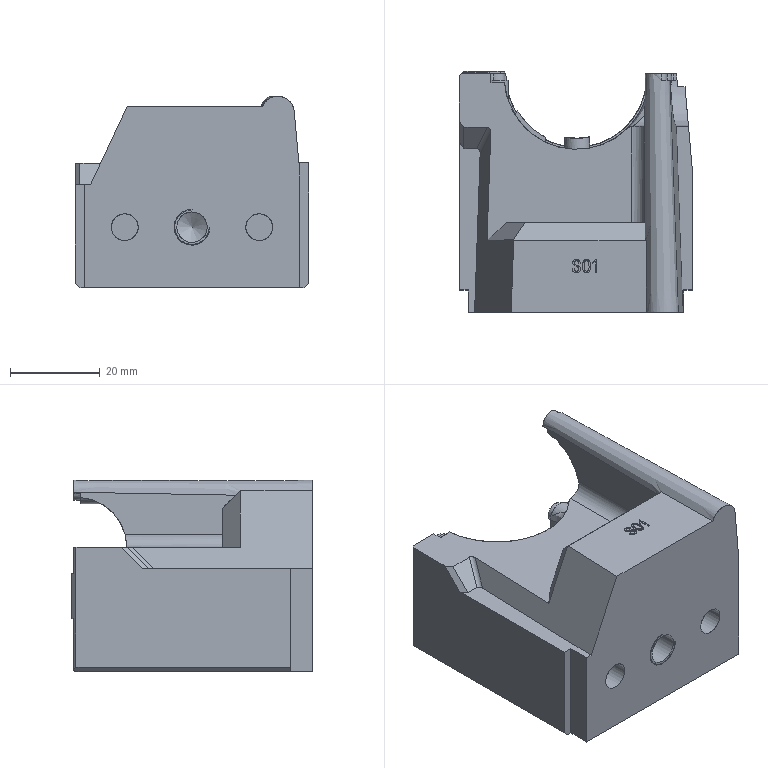NC program | PowerMill | posted with a generic post | part box 52 x 53.756 x 42.711 mm
Lines 1 to 741 of 2084:
%
O0001
N104 ( POWERMILL CB  : 2026004.0)
N105 ( POST VER      : 2026.0.0.5161)
N106 ( OPTION FILE   : FANUC)
N107 ( OUTPUT WORKPLANE : 3)
N108 (  )
N109 ( TOOL LIST )
N110 (----------------------------------)
N111 ( NO. | ID   | DIA.| TIP RAD|LENGTH)
N112 (----------------------------------)
N113 (    1|D4_1_1| 4.0 |  0.0   |108.56)
N114 (----------------------------------)
N115 (  )
N116 ( NUMBER OF TOOLPATHS: 1.0 )
N117 ( ESTIMATED PROGRAM DURATION: 0 HOURS 0 MIN 30 SEC)
N118 (  )
N119 G00 G21 G80 G40 G17
N120 G90
N121 G54
N122 G53 Z0.0
N123 (---------------)
N124 ( START TOOLPATH : 18开粗-D4-等高 )
N125 (---------------)
N126 ( TOOL NO.    :1 )
N127 ( TOOL TYPE   : ENDMILL)
N128 ( TOOL ID     : D4_1_1)
N129 ( TOOL DIA    : 4.0 LENGTH 108.56)
N130 T1
N131 M6
N132 S5500 M03
N133 G00 G90 X-25.2597 Y38.9756
N134 G43 Z63.21 H1
N135
N136 G05 P10000 R8
N137 Z30.842
N138 G01 Z27.842 F1800.0
N139 G02 X-24.8595 Y39.082 I0.3987 J-0.6936 F3000.0
N140 G01 X-21.6418 Y39.0761
N141 G02 X-21.2418 Y38.6655 I0.0002 J-0.4
N142 G01 X-21.362 Y35.186
N143 G02 X-21.483 Y34.7899 I-0.7996 J0.0276
N144 G01 X-21.512 Y34.7433
N145 X-21.5257 Y34.7207 Z27.8377
N146 X-21.5374 Y34.7001 Z27.8252
N147 X-21.5582 Y34.6616 Z27.7921
N148 X-21.561 Y34.6521 Z27.7611
N149 X-21.5457 Y34.6737 Z27.7422
N150 G03 X-21.4246 Y35.0697 I-0.6784 J0.4239
N151 G01 X-21.3028 Y38.5581
N152 G03 X-21.7026 Y38.9721 I-0.3998 J0.014
N153 G01 X-24.9911 Y38.9748
N154 G03 X-25.3912 Y38.8679 I-0.0006 J-0.8
N155 G01 X-25.4333 Y38.8436
N156 X-25.4578 Y38.8268 Z27.7371
N157 X-25.4764 Y38.8082 Z27.7225
N158 X-25.5002 Y38.7783 Z27.6923
N159 X-25.4996 Y38.7617 Z27.6607
N160 X-25.4697 Y38.7691 Z27.6424
N161 G02 X-25.0696 Y38.8758 I0.3992 J-0.6932
N162 G01 X-21.7526 Y38.8723
N163 G02 X-21.3529 Y38.4583 I0.0 J-0.4
N164 G01 X-21.4751 Y34.9589
N165 G02 X-21.5961 Y34.5629 I-0.7995 J0.0279
N166 G01 X-21.621 Y34.523
N167 X-21.6348 Y34.4999 Z27.6375
N168 X-21.6458 Y34.4792 Z27.6235
N169 X-21.6613 Y34.4474 Z27.5925
N170 X-21.6623 Y34.4389 Z27.5611
N171 X-21.6463 Y34.4605 Z27.5426
N172 G03 X-21.5252 Y34.8565 I-0.6784 J0.4239
N173 G01 X-21.4029 Y38.3585
N174 G03 X-21.8027 Y38.7725 I-0.3998 J0.014
N175 G01 X-25.1457 Y38.778
N176 G03 X-25.5459 Y38.6715 I-0.0013 J-0.8
N177 G01 X-25.5709 Y38.6571
N178 X-25.5973 Y38.6444 Z27.5356
N179 X-25.6195 Y38.6384 Z27.5163
N180 X-25.6379 Y38.6364 Z27.4921
N181 X-25.6424 Y38.641 Z27.4598
N182 X-25.6171 Y38.6535 Z27.4428
N183 G02 X-25.2045 Y38.689 I0.2727 J-0.7521
N184 G01 X-25.1367 Y38.677
N185 X-21.8527 Y38.6727
N186 G02 X-21.4529 Y38.2587 I0.0 J-0.4
N187 G01 X-21.5753 Y34.7559
N188 G02 X-21.6963 Y34.3599 I-0.7995 J0.0279
N189 G01 X-21.7209 Y34.3205
N190 X-21.7347 Y34.2975 Z27.4379
N191 X-21.7458 Y34.2769 Z27.4237
N192 X-21.7612 Y34.2458 Z27.3929
N193 X-21.7624 Y34.2375 Z27.3614
N194 X-21.7464 Y34.2592 Z27.343
N195 G03 X-21.6253 Y34.6552 I-0.6785 J0.424
N196 G01 X-21.503 Y38.1589
N197 G03 X-21.9028 Y38.5729 I-0.3997 J0.014
N198 G01 X-25.1367 Y38.5772
N199 X-25.2536 Y38.5993
N200 G03 X-25.6665 Y38.5684 I-0.1488 J-0.786
N201 G01 X-25.6952 Y38.5584
N202 X-25.7259 Y38.5425 Z27.3355
N203 X-25.7455 Y38.5215 Z27.3149
N204 X-25.7556 Y38.5031 Z27.2933
N205 X-25.749 Y38.4824 Z27.26
N206 X-25.713 Y38.483 Z27.2433
N207 G02 X-25.2997 Y38.5099 I0.2568 J-0.7577
N208 G01 X-25.1367 Y38.4774
N209 X-21.9528 Y38.4731
N210 G02 X-21.553 Y38.0591 I0.0 J-0.4
N211 G01 X-21.6754 Y34.5561
N212 G02 X-21.7964 Y34.16 I-0.7995 J0.0279
N213 G01 X-21.8206 Y34.1215
N214 X-21.8344 Y34.0984 Z27.2382
N215 X-21.8455 Y34.078 Z27.2239
N216 X-21.8608 Y34.0479 Z27.1934
N217 X-21.8622 Y34.04 Z27.1618
N218 X-21.8464 Y34.0618 Z27.1435
N219 G03 X-21.7254 Y34.4578 I-0.6785 J0.424
N220 G01 X-21.6031 Y37.9593
N221 G03 X-22.0028 Y38.3733 I-0.3997 J0.014
N222 G01 X-25.1367 Y38.3776
N223 X-25.3471 Y38.4066
N224 G03 X-25.758 Y38.3551 I-0.1092 J-0.7925
N225 G01 X-25.784 Y38.3445
N226 X-25.8136 Y38.3273 Z27.1356
N227 X-25.8316 Y38.3059 Z27.1142
N228 X-25.8395 Y38.2893 Z27.0938
N229 X-25.8315 Y38.2701 Z27.0603
N230 X-25.7959 Y38.2728 Z27.0437
N231 G02 X-25.3841 Y38.3167 I0.2877 J-0.7464
N232 G01 X-25.1367 Y38.2778
N233 X-22.0529 Y38.2735
N234 G02 X-21.6531 Y37.8596 I0.0 J-0.4
N235 G01 X-21.7754 Y34.3596
N236 G02 X-21.8964 Y33.9636 I-0.7995 J0.028
N237 G01 X-21.9203 Y33.9254
N238 X-21.9342 Y33.9023 Z27.0386
N239 X-21.9454 Y33.8819 Z27.0242
N240 X-21.9606 Y33.8523 Z26.9938
N241 X-21.962 Y33.8446 Z26.9622
N242 X-21.9464 Y33.8665 Z26.9439
N243 G03 X-21.8253 Y34.2625 I-0.6784 J0.4239
N244 G01 X-21.7032 Y37.7598
N245 G03 X-22.1029 Y38.1737 I-0.3997 J0.0139
N246 G01 X-25.1367 Y38.178
N247 X-25.4225 Y38.2229
N248 G03 X-25.8343 Y38.179 I-0.1241 J-0.7904
N249 G01 X-25.8618 Y38.1685
N250 X-25.8932 Y38.1501 Z26.936
N251 X-25.9119 Y38.126 Z26.9147
N252 X-25.9198 Y38.1066 Z26.894
N253 X-25.9106 Y38.0838 Z26.8607
N254 X-25.8727 Y38.0853 Z26.8441
N255 G02 X-25.4609 Y38.1291 I0.2877 J-0.7465
N256 G01 X-25.1367 Y38.0782
N257 X-22.153 Y38.0739
N258 G02 X-21.7532 Y37.66 I0.0 J-0.4
N259 G01 X-21.8752 Y34.1663
N260 G02 X-21.9963 Y33.7703 I-0.7995 J0.0279
N261 G01 X-22.02 Y33.7323
N262 X-22.0339 Y33.7093 Z26.839
N263 X-22.0451 Y33.6889 Z26.8245
N264 X-22.0603 Y33.6597 Z26.7942
N265 X-22.0618 Y33.6521 Z26.7626
N266 X-22.0462 Y33.674 Z26.7443
N267 G03 X-21.9252 Y34.0701 I-0.6785 J0.424
N268 G01 X-21.8033 Y37.5602
N269 G03 X-22.203 Y37.9741 I-0.3997 J0.0139
N270 G01 X-25.1367 Y37.9784
N271 X-25.4875 Y38.0333
N272 G03 X-25.8993 Y37.9892 I-0.1236 J-0.7904
N273 G01 X-25.9238 Y37.9797
N274 X-25.9562 Y37.9601 Z26.7358
N275 X-25.974 Y37.9342 Z26.713
N276 X-25.9795 Y37.9165 Z26.6944
N277 X-25.9679 Y37.8929 Z26.6608
N278 X-25.9284 Y37.8945 Z26.6445
N279 G02 X-25.5167 Y37.9383 I0.2877 J-0.7465
N280 G01 X-25.1367 Y37.8786
N281 X-22.2531 Y37.8743
N282 G02 X-21.8533 Y37.4604 I0.0 J-0.4
N283 G01 X-21.9751 Y33.9738
N284 G02 X-22.0962 Y33.5778 I-0.7995 J0.0279
N285 G01 X-22.1199 Y33.5398
N286 X-22.1338 Y33.5168 Z26.6394
N287 X-22.145 Y33.4965 Z26.6249
N288 X-22.1602 Y33.4672 Z26.5946
N289 X-22.1617 Y33.4596 Z26.563
N290 X-22.1461 Y33.4816 Z26.5447
N291 G03 X-22.025 Y33.8776 I-0.6785 J0.4239
N292 G01 X-21.9035 Y37.3606
N293 G03 X-22.3033 Y37.7746 I-0.3998 J0.014
N294 G01 X-25.1367 Y37.7789
N295 X-25.5407 Y37.8433
N296 G03 X-25.9526 Y37.8004 I-0.126 J-0.7901
N297 G01 X-25.9741 Y37.7922
N298 X-26.0063 Y37.773 Z26.5357
N299 X-26.0232 Y37.7479 Z26.5118
N300 X-26.0272 Y37.7334 Z26.495
N301 X-26.015 Y37.7116 Z26.461
N302 X-25.9761 Y37.7135 Z26.4449
N303 G02 X-25.5637 Y37.7519 I0.2779 J-0.7503
N304 G01 X-25.1367 Y37.6791
N305 X-22.3532 Y37.6748
N306 G02 X-21.9534 Y37.2608 I0.0 J-0.4
N307 G01 X-22.0749 Y33.7814
N308 G02 X-22.196 Y33.3853 I-0.7995 J0.0279
N309 G01 X-22.2196 Y33.3475
N310 X-22.2335 Y33.3245 Z26.4398
N311 X-22.2448 Y33.3042 Z26.4253
N312 X-22.2599 Y33.2751 Z26.395
N313 X-22.2615 Y33.2676 Z26.3634
N314 X-22.2459 Y33.2896 Z26.3451
N315 G03 X-22.1248 Y33.6856 I-0.6784 J0.4239
N316 G01 X-22.0035 Y37.161
N317 G03 X-22.4032 Y37.575 I-0.3997 J0.014
N318 G01 X-25.1367 Y37.5793
N319 X-25.4545 Y37.6235
N320 X-25.5837 Y37.6596
N321 G03 X-25.9978 Y37.6641 I-0.2154 J-0.7704
N322 G01 X-26.0194 Y37.6586
N323 X-26.0644 Y37.6335 Z26.3353
N324 X-26.0854 Y37.5929 Z26.3097
N325 X-26.0882 Y37.5701 Z26.2936
N326 X-26.0685 Y37.5327 Z26.2608
N327 X-26.0174 Y37.5301 Z26.2453
N328 G02 X-25.6047 Y37.5643 I0.2701 J-0.753
N329 G01 X-25.1367 Y37.4795
N330 X-22.4533 Y37.4752
N331 G02 X-22.0535 Y37.0612 I0.0 J-0.4
N332 G01 X-22.1747 Y33.5917
N333 G02 X-22.2957 Y33.1957 I-0.7995 J0.0279
N334 G01 X-22.319 Y33.1584
N335 X-22.333 Y33.1354 Z26.2402
N336 X-22.3443 Y33.1152 Z26.2255
N337 X-22.3593 Y33.0869 Z26.1954
N338 X-22.361 Y33.0796 Z26.1638
N339 X-22.3456 Y33.1017 Z26.1455
N340 G03 X-22.2245 Y33.4978 I-0.6784 J0.424
N341 G01 X-22.1036 Y36.9614
N342 G03 X-22.5033 Y37.3754 I-0.3997 J0.014
N343 G01 X-25.1367 Y37.3797
N344 X-25.5357 Y37.4423
N345 X-25.6217 Y37.4749
N346 G03 X-26.0337 Y37.5165 I-0.2836 J-0.748
N347 G01 X-26.0486 Y37.5141
N348 X-26.0888 Y37.4978 Z26.1347
N349 X-26.1089 Y37.4694 Z26.1066
N350 X-26.111 Y37.4592 Z26.0956
N351 X-26.0965 Y37.4306 Z26.0612
N352 X-26.0526 Y37.4239 Z26.0457
N353 G02 X-25.6405 Y37.3823 I0.1284 J-0.7897
N354 G01 X-25.5357 Y37.3425
N355 X-25.1367 Y37.2799
N356 X-22.5534 Y37.2756
N357 G02 X-22.1536 Y36.8616 I0.0 J-0.4
N358 G01 X-22.2744 Y33.4038
N359 G02 X-22.3954 Y33.0078 I-0.7995 J0.028
N360 G01 X-22.4186 Y32.9708
N361 X-22.4325 Y32.9477 Z26.0406
N362 X-22.4439 Y32.9276 Z26.0258
N363 X-22.4589 Y32.8996 Z25.9959
N364 X-22.4606 Y32.8925 Z25.9642
N365 X-22.4452 Y32.9146 Z25.946
N366 G03 X-22.3242 Y33.3106 I-0.6785 J0.4239
N367 G01 X-22.2037 Y36.7618
N368 G03 X-22.6034 Y37.1758 I-0.3997 J0.014
N369 G01 X-25.1367 Y37.1801
N370 X-25.4553 Y37.2245
N371 X-25.6594 Y37.2896
N372 G03 X-26.073 Y37.3092 I-0.2432 J-0.7621
N373 G01 X-26.0914 Y37.3052
N374 X-26.1306 Y37.287 Z25.9358
N375 X-26.1506 Y37.2576 Z25.9092
N376 X-26.1534 Y37.2445 Z25.8961
N377 X-26.1391 Y37.2153 Z25.8618
N378 X-26.0948 Y37.21 Z25.8462
N379 G02 X-25.6812 Y37.1897 I0.1689 J-0.782
N380 G01 X-25.5357 Y37.1429
N381 X-25.1367 Y37.0803
N382 X-22.6535 Y37.076
N383 G02 X-22.2537 Y36.662 I0.0 J-0.4
N384 G01 X-22.374 Y33.2184
N385 G02 X-22.495 Y32.8224 I-0.7995 J0.0279
N386 G01 X-22.518 Y32.7856
N387 X-22.532 Y32.7626 Z25.841
N388 X-22.5434 Y32.7425 Z25.8262
N389 X-22.5583 Y32.7149 Z25.7963
N390 X-22.5601 Y32.7079 Z25.7646
N391 X-22.5448 Y32.7301 Z25.7464
N392 G03 X-22.4238 Y33.1261 I-0.6785 J0.4239
N393 G01 X-22.3039 Y36.5623
N394 G03 X-22.7037 Y36.9762 I-0.3998 J0.0139
N395 G01 X-25.1367 Y36.9805
N396 X-25.5357 Y37.0432
N397 X-25.697 Y37.1043
N398 G03 X-26.1091 Y37.1459 I-0.2837 J-0.748
N399 G01 X-26.124 Y37.1435
N400 X-26.1642 Y37.1272 Z25.7355
N401 X-26.1842 Y37.0988 Z25.7075
N402 X-26.1863 Y37.0886 Z25.6965
N403 X-26.1718 Y37.06 Z25.662
N404 X-26.1279 Y37.0533 Z25.6466
N405 G02 X-25.7159 Y37.0117 I0.1284 J-0.7897
N406 G01 X-25.5357 Y36.9434
N407 X-25.1367 Y36.8807
N408 X-22.7536 Y36.8764
N409 G02 X-22.3538 Y36.4625 I0.0001 J-0.4
N410 G01 X-22.4735 Y33.0339
N411 G02 X-22.5946 Y32.6379 I-0.7995 J0.0279
N412 G01 X-22.6172 Y32.6016
N413 X-22.6313 Y32.5786 Z25.6413
N414 X-22.6427 Y32.5586 Z25.6264
N415 X-22.6575 Y32.5317 Z25.5967
N416 X-22.6595 Y32.525 Z25.5649
N417 X-22.6443 Y32.5473 Z25.5468
N418 G03 X-22.5232 Y32.9434 I-0.6785 J0.424
N419 G01 X-22.4038 Y36.3627
N420 G03 X-22.8036 Y36.7766 I-0.3998 J0.0139
N421 G01 X-25.1367 Y36.7809
N422 X-25.4561 Y36.8255
N423 X-25.7347 Y36.919
N424 G03 X-26.148 Y36.9447 I-0.2546 J-0.7584
N425 G01 X-26.1673 Y36.9409
N426 X-26.2088 Y36.9217 Z25.5366
N427 X-26.2299 Y36.8894 Z25.5101
N428 X-26.233 Y36.8746 Z25.4967
N429 X-26.2178 Y36.8419 Z25.4626
N430 X-26.1712 Y36.8355 Z25.447
N431 G02 X-25.7576 Y36.8151 I0.1687 J-0.782
N432 G01 X-25.5357 Y36.7438
N433 X-25.1367 Y36.6811
N434 X-22.8536 Y36.6768
N435 G02 X-22.4539 Y36.2629 I0.0 J-0.4
N436 G01 X-22.573 Y32.8528
N437 G02 X-22.694 Y32.4568 I-0.7995 J0.028
N438 G01 X-22.7167 Y32.4206
N439 X-22.7307 Y32.3976 Z25.4418
N440 X-22.7422 Y32.3776 Z25.4268
N441 X-22.757 Y32.3507 Z25.3971
N442 X-22.7589 Y32.344 Z25.3653
N443 X-22.7438 Y32.3663 Z25.3472
N444 G03 X-22.6227 Y32.7623 I-0.6784 J0.424
N445 G01 X-22.5039 Y36.1631
N446 G03 X-22.9037 Y36.577 I-0.3998 J0.014
N447 G01 X-25.1367 Y36.5813
N448 X-25.5357 Y36.644
N449 X-25.7724 Y36.7337
N450 G03 X-26.1844 Y36.7753 I-0.2836 J-0.748
N451 G01 X-26.1993 Y36.7729
N452 X-26.2395 Y36.7566 Z25.3363
N453 X-26.2596 Y36.7282 Z25.3083
N454 X-26.2617 Y36.718 Z25.2973
N455 X-26.2472 Y36.6894 Z25.2629
N456 X-26.2032 Y36.6827 Z25.2474
N457 G02 X-25.7912 Y36.6411 I0.1283 J-0.7897
N458 G01 X-25.5357 Y36.5442
N459 X-25.1367 Y36.4816
N460 X-22.9537 Y36.4773
N461 G02 X-22.554 Y36.0633 I0.0 J-0.4
N462 G01 X-22.6724 Y32.6726
N463 G02 X-22.7935 Y32.2765 I-0.7995 J0.0279
N464 G01 X-22.8158 Y32.2408
N465 X-22.8299 Y32.2177 Z25.2421
N466 X-22.8414 Y32.1979 Z25.227
N467 X-22.8561 Y32.1715 Z25.1975
N468 X-22.8582 Y32.1651 Z25.1657
N469 X-22.8431 Y32.1875 Z25.1476
N470 G03 X-22.7221 Y32.5835 I-0.6785 J0.4239
N471 G01 X-22.604 Y35.9635
N472 G03 X-23.0038 Y36.3775 I-0.3998 J0.014
N473 G01 X-25.1367 Y36.3818
N474 X-25.457 Y36.4265
N475 X-25.8101 Y36.5484
N476 G03 X-26.2232 Y36.5777 I-0.2611 J-0.7561
N477 G01 X-26.2411 Y36.5742
N478 X-26.2825 Y36.5556 Z25.1372
N479 X-26.3033 Y36.5239 Z25.1102
N480 X-26.306 Y36.5105 Z25.0976
N481 X-26.2907 Y36.4786 Z25.0634
N482 X-26.2445 Y36.4719 Z25.0478
N483 G02 X-25.8313 Y36.4449 I0.1562 J-0.7846
N484 G01 X-25.5357 Y36.3446
N485 X-25.1367 Y36.282
N486 X-23.0538 Y36.2777
N487 G02 X-22.6541 Y35.8637 I0.0 J-0.4
N488 G01 X-22.7717 Y32.4945
N489 G02 X-22.8928 Y32.0985 I-0.7995 J0.0279
N490 G01 X-22.9152 Y32.0627
N491 X-22.9292 Y32.0397 Z25.0425
N492 X-22.9408 Y32.0198 Z25.0274
N493 X-22.9555 Y31.9935 Z24.9979
N494 X-22.9576 Y31.987 Z24.9661
N495 X-22.9425 Y32.0094 Z24.948
N496 G03 X-22.8214 Y32.4055 I-0.6785 J0.424
N497 G01 X-22.7043 Y35.7639
N498 G03 X-23.104 Y36.1779 I-0.3997 J0.014
N499 G01 X-25.1367 Y36.1822
N500 X-25.5357 Y36.2448
N501 X-25.8478 Y36.3632
N502 G03 X-26.2598 Y36.4047 I-0.2836 J-0.7481
N503 G01 X-26.2747 Y36.4023
N504 X-26.3149 Y36.386 Z24.9372
N505 X-26.335 Y36.3576 Z24.9091
N506 X-26.3371 Y36.3474 Z24.8981
N507 X-26.3226 Y36.3188 Z24.8637
N508 X-26.2786 Y36.3121 Z24.8482
N509 G02 X-25.8666 Y36.2705 I0.1284 J-0.7896
N510 G01 X-25.5357 Y36.145
N511 X-25.1367 Y36.0824
N512 X-23.1539 Y36.0779
N513 G02 X-22.7542 Y35.664 I0.0 J-0.4
N514 G01 X-22.871 Y32.3174
N515 G02 X-22.9921 Y31.9214 I-0.7996 J0.0279
N516 G01 X-23.0143 Y31.8859
N517 X-23.0284 Y31.8629 Z24.8429
N518 X-23.0399 Y31.8431 Z24.8277
N519 X-23.0546 Y31.8171 Z24.7983
N520 X-23.0568 Y31.8109 Z24.7665
N521 X-23.0418 Y31.8334 Z24.7485
N522 G03 X-22.9207 Y32.2294 I-0.6784 J0.4239
N523 G01 X-22.8042 Y35.5643
N524 G03 X-23.204 Y35.9783 I-0.3998 J0.014
N525 G01 X-25.1367 Y35.9826
N526 X-25.4578 Y36.0275
N527 X-25.8855 Y36.1779
N528 G03 X-26.2984 Y36.2094 I-0.2653 J-0.7547
N529 G01 X-26.3146 Y36.2064
N530 X-26.3544 Y36.1892 Z24.7378
N531 X-26.3744 Y36.1603 Z24.7103
N532 X-26.3767 Y36.1493 Z24.6987
N533 X-26.3621 Y36.1203 Z24.6642
N534 X-26.3179 Y36.114 Z24.6487
N535 G02 X-25.9052 Y36.0789 I0.1409 J-0.7875
N536 G01 X-25.5357 Y35.9454
N537 X-25.1367 Y35.8828
N538 X-23.254 Y35.8785
N539 G02 X-22.8543 Y35.4645 I0.0 J-0.4
N540 G01 X-22.9703 Y32.1414
N541 G02 X-23.0914 Y31.7453 I-0.7995 J0.0279
N542 G01 X-23.1135 Y31.7099
N543 X-23.1277 Y31.6868 Z24.6433
N544 X-23.1392 Y31.667 Z24.6281
N545 X-23.1538 Y31.6411 Z24.5988
N546 X-23.156 Y31.6349 Z24.5669
N547 X-23.141 Y31.6573 Z24.5489
N548 G03 X-23.0199 Y32.0533 I-0.6785 J0.424
N549 G01 X-22.9043 Y35.3647
N550 G03 X-23.3041 Y35.7787 I-0.3998 J0.014
N551 G01 X-25.1367 Y35.783
N552 X-25.5357 Y35.8456
N553 X-25.9234 Y35.9927
N554 G03 X-26.3354 Y36.0343 I-0.2836 J-0.748
N555 G01 X-26.3505 Y36.0318
N556 X-26.3906 Y36.0156 Z24.538
N557 X-26.4107 Y35.9872 Z24.5101
N558 X-26.4128 Y35.977 Z24.499
N559 X-26.3984 Y35.9485 Z24.4645
N560 X-26.3546 Y35.9417 Z24.4491
N561 G02 X-25.9426 Y35.9001 I0.1284 J-0.7896
N562 G01 X-25.5357 Y35.7459
N563 X-25.1367 Y35.6832
N564 X-23.3541 Y35.6789
N565 G02 X-22.9544 Y35.265 I0.0 J-0.4
N566 G01 X-23.0696 Y31.9657
N567 G02 X-23.1906 Y31.5697 I-0.7995 J0.0279
N568 G01 X-23.2122 Y31.5352
N569 X-23.2264 Y31.5122 Z24.4436
N570 X-23.2381 Y31.4925 Z24.4282
N571 X-23.2525 Y31.4679 Z24.3992
N572 X-23.255 Y31.4622 Z24.3673
N573 X-23.2402 Y31.4848 Z24.3493
N574 G03 X-23.1191 Y31.8808 I-0.6784 J0.424
N575 G01 X-23.0044 Y35.1652
N576 G03 X-23.4042 Y35.5791 I-0.3998 J0.0139
N577 G01 X-25.1367 Y35.5834
N578 X-25.4589 Y35.6285
N579 X-25.9618 Y35.8076
N580 G03 X-26.3746 Y35.8409 I-0.2684 J-0.7536
N581 G01 X-26.3862 Y35.8387
N582 X-26.4213 Y35.8262 Z24.3379
N583 X-26.4388 Y35.8073 Z24.3086
N584 X-26.4401 Y35.8027 Z24.3004
N585 X-26.4277 Y35.7845 Z24.265
N586 X-26.3894 Y35.7799 Z24.2495
N587 G02 X-25.9806 Y35.7136 I0.0807 J-0.7959
N588 G01 X-25.7915 Y35.6285
N589 X-25.5357 Y35.5463
N590 X-25.1367 Y35.4836
N591 X-23.4542 Y35.4793
N592 G02 X-23.0545 Y35.0654 I0.0 J-0.4
N593 G01 X-23.1686 Y31.796
N594 G02 X-23.2897 Y31.3999 I-0.7995 J0.0279
N595 G01 X-23.3093 Y31.3686
N596 X-23.3239 Y31.3455 Z24.2437
N597 X-23.3362 Y31.3266 Z24.2272
N598 X-23.3497 Y31.306 Z24.1996
N599 X-23.353 Y31.3022 Z24.1674
N600 X-23.3389 Y31.3256 Z24.1497
N601 G03 X-23.2178 Y31.7216 I-0.6784 J0.4239
N602 G01 X-23.1046 Y34.9656
N603 G03 X-23.5044 Y35.3795 I-0.3998 J0.0139
N604 G01 X-25.1367 Y35.3838
N605 X-25.5357 Y35.4465
N606 X-26.0 Y35.6225
N607 G03 X-26.412 Y35.6641 I-0.2836 J-0.748
N608 G01 X-26.4195 Y35.6629
N609 X-26.4639 Y35.6429 Z24.137
N610 X-26.4817 Y35.6083 Z24.1052
N611 Y35.6029 Z24.0998
N612 X-26.4608 Y35.5714 Z24.0649
N613 X-26.412 Y35.5643 Z24.0499
N614 G02 X-26.0 Y35.5227 I0.1284 J-0.7896
N615 G01 X-25.5357 Y35.3467
N616 X-25.1367 Y35.284
N617 X-23.5543 Y35.2798
N618 G02 X-23.1545 Y34.8658 I0.0 J-0.4
N619 G01 X-23.2668 Y31.6525
N620 G02 X-23.3878 Y31.2565 I-0.7995 J0.0279
N621 G01 X-23.4064 Y31.2267
N622 X-23.4213 Y31.2035 Z24.0438
N623 X-23.4339 Y31.1849 Z24.0268
N624 X-23.447 Y31.1664 Z24.0
N625 X-23.4507 Y31.1635 Z23.9677
N626 X-23.4368 Y31.1873 Z23.9501
N627 G03 X-23.3157 Y31.5834 I-0.6785 J0.424
N628 G01 X-23.2046 Y34.766
N629 G03 X-23.6044 Y35.18 I-0.3997 J0.014
N630 G01 X-25.1367 Y35.1843
N631 X-25.4593 Y35.2295
N632 X-26.0 Y35.423
N633 G03 X-26.4127 Y35.4568 I-0.2695 J-0.7534
N634 G01 X-26.4166 Y35.4561
N635 X-26.4556 Y35.4402 Z23.9364
N636 X-26.4704 Y35.416 Z23.9025
N637 Y35.4153 Z23.9013
N638 X-26.4516 Y35.3945 Z23.8653
N639 X-26.4088 Y35.3893 Z23.8503
N640 G02 X-26.0 Y35.3232 I0.0809 J-0.7959
N641 G01 X-25.7916 Y35.2295
N642 X-25.5357 Y35.1471
N643 X-25.1367 Y35.0845
N644 X-23.6544 Y35.0802
N645 G02 X-23.2546 Y34.6662 I0.0 J-0.4
N646 G01 X-23.3647 Y31.5142
N647 G02 X-23.4858 Y31.1182 I-0.7995 J0.028
N648 G01 X-23.5012 Y31.0936
N649 X-23.517 Y31.07 Z23.8434
N650 X-23.5309 Y31.0528 Z23.8241
N651 X-23.5424 Y31.0406 Z23.8004
N652 X-23.5472 Y31.0413 Z23.7676
N653 X-23.5341 Y31.0667 Z23.7505
N654 G03 X-23.4131 Y31.4627 I-0.6785 J0.4239
N655 G01 X-23.3047 Y34.5664
N656 G03 X-23.7044 Y34.9804 I-0.3997 J0.014
N657 G01 X-25.1367 Y34.9847
N658 X-25.5357 Y35.0473
N659 X-26.0 Y35.2234
N660 G03 X-26.412 Y35.265 I-0.2836 J-0.748
N661 G01 X-26.4195 Y35.2637
N662 X-26.4639 Y35.2438 Z23.7378
N663 X-26.4817 Y35.2091 Z23.706
N664 Y35.2037 Z23.7006
N665 X-26.4608 Y35.1722 Z23.6657
N666 X-26.412 Y35.1652 Z23.6507
N667 G02 X-26.0 Y35.1236 I0.1284 J-0.7896
N668 G01 X-25.5357 Y34.9475
N669 X-25.1367 Y34.8849
N670 X-23.7544 Y34.8804
N671 G02 X-23.3547 Y34.4665 I-0.0001 J-0.4
N672 G01 X-23.4601 Y31.4504
N673 G02 X-23.5811 Y31.0544 I-0.7995 J0.0279
N674 G01 X-23.5873 Y31.0445
N675 X-23.609 Y31.0179 Z23.6397
N676 X-23.6287 Y31.0072 Z23.6114
N677 X-23.6336 Y31.0071 Z23.6008
N678 X-23.6407 Y31.0211 Z23.5664
N679 X-23.6277 Y31.0532 Z23.5509
N680 G03 X-23.5067 Y31.4492 I-0.6785 J0.424
N681 G01 X-23.4048 Y34.3668
N682 G03 X-23.8045 Y34.7808 I-0.3997 J0.014
N683 G01 X-25.1367 Y34.7851
N684 X-25.4601 Y34.8305
N685 X-26.0 Y35.0238
N686 G03 X-26.4127 Y35.0577 I-0.2696 J-0.7532
N687 G01 X-26.4166 Y35.057
N688 X-26.4556 Y35.0411 Z23.5372
N689 X-26.4705 Y35.0169 Z23.5033
N690 X-26.4704 Y35.0161 Z23.5021
N691 X-26.4516 Y34.9952 Z23.4662
N692 X-26.4088 Y34.9901 Z23.4512
N693 G02 X-26.0 Y34.924 I0.0811 J-0.7959
N694 G01 X-25.7919 Y34.8305
N695 X-25.5357 Y34.7479
N696 X-25.1367 Y34.6853
N697 X-23.8546 Y34.681
N698 G02 X-23.4548 Y34.267 I0.0 J-0.4
N699 G01 X-23.5533 Y31.448
N700 G02 X-23.6743 Y31.052 I-0.7995 J0.028
N701 G01 X-23.6805 Y31.0421
N702 X-23.7022 Y31.0155 Z23.4401
N703 X-23.7219 Y31.0049 Z23.4118
N704 X-23.7268 Y31.0047 Z23.4013
N705 X-23.7339 Y31.0187 Z23.3668
N706 X-23.721 Y31.0508 Z23.3514
N707 G03 X-23.5999 Y31.4469 I-0.6784 J0.424
N708 G01 X-23.5049 Y34.1672
N709 G03 X-23.9046 Y34.5812 I-0.3997 J0.014
N710 G01 X-25.1367 Y34.5855
N711 X-25.5357 Y34.6481
N712 X-25.9996 Y34.824
N713 G03 X-26.4117 Y34.8656 I-0.2836 J-0.7481
N714 G01 X-26.4171 Y34.8647
N715 X-26.463 Y34.8434 Z23.3381
N716 X-26.4801 Y34.8065 Z23.3053
N717 X-26.4799 Y34.8025 Z23.3014
N718 X-26.457 Y34.7697 Z23.2664
N719 X-26.4065 Y34.7625 Z23.2516
N720 G02 X-25.9944 Y34.7215 I0.1295 J-0.7894
N721 G01 X-25.5357 Y34.5484
N722 X-25.1367 Y34.4857
N723 X-23.9547 Y34.4814
N724 G02 X-23.5549 Y34.0675 I0.0 J-0.4
N725 G01 X-23.6465 Y31.4457
N726 G02 X-23.7676 Y31.0497 I-0.7995 J0.0279
N727 G01 X-23.7732 Y31.0406
N728 X-23.7942 Y31.015 Z23.2409
N729 X-23.8133 Y31.005 Z23.2135
N730 X-23.8178 Z23.2038
N731 X-23.8246 Y31.0189 Z23.1707
N732 X-23.8121 Y31.0498 Z23.156
N733 G03 X-23.6911 Y31.4458 I-0.6785 J0.424
N734 G01 X-23.6029 Y33.9719
N735 G03 X-24.0026 Y34.3858 I-0.3997 J0.0139
N736 G01 X-25.1367 Y34.3901
N737 X-25.5357 Y34.4528
N738 X-25.9927 Y34.6251
N739 G03 X-26.4048 Y34.6659 I-0.2822 J-0.7485
N740 G00 Z46.7139
N741 G01 X13.5473 Y17.4207 F10000.0
N742 G00 Z44.0146
N743 G01 Z41.0146 F1800.0
N744 G03 X13.6517 Y17.8215 I-0.6956 J0.3951 F3000.0
N745 G01 X13.6288 Y21.0678
N746 G03 X13.5188 Y21.467 I-0.8 J-0.0057
N747 G01 X13.4312 Y21.6164
N748 X13.4096 Y21.6631 Z41.0116
N749 X13.398 Y21.7126 Z41.0029
N750 X13.3766 Y21.8801 Z40.9647
N751 X13.4065 Y21.9302 Z40.9351
N752 X13.4628 Y21.9038 Z40.9148
N753 G02 X13.5728 Y21.5046 I-0.69 J-0.4049
N754 G01 X13.5994 Y17.734
N755 G02 X13.495 Y17.3332 I-0.8 J-0.0056
N756 G01 X13.4796 Y17.3061
N757 X13.4646 Y17.282 Z40.9081
N758 X13.4507 Y17.2642 Z40.8896
N759 X13.4376 Y17.2502 Z40.8649
N760 X13.4311 Y17.2507 Z40.8322
N761 X13.4425 Y17.2768 Z40.815
N762 G03 X13.5472 Y17.6775 I-0.6953 J0.3957
N763 G01 X13.522 Y21.7136
N764 G03 X13.4123 Y22.1129 I-0.8 J-0.005
N765 G01 X13.3833 Y22.1626
N766 X13.3705 Y22.1875 Z40.8106
N767 X13.3617 Y22.2114 Z40.798
N768 X13.3489 Y22.2568 Z40.7651
N769 X13.3534 Y22.271 Z40.7341
N770 X13.3734 Y22.2503 Z40.7152
N771 G02 X13.4827 Y21.8508 I-0.6907 J-0.4037
N772 G01 X13.5049 Y17.6251
N773 G02 X13.3999 Y17.2245 I-0.7999 J-0.0042
N774 G00 Z46.3709
N775 G01 X9.4078 Y18.2716 F10000.0
N776 G00 Z43.6154
N777 G01 Z40.6154 F1800.0
N778 G03 X9.8077 Y18.1639 I0.401 J0.6923 F3000.0
N779 G01 X13.059 Y18.1594
N780 G03 X13.459 Y18.5616 I0.0 J0.4
N781 G01 X13.4404 Y21.9836
N782 G03 X13.3311 Y22.383 I-0.8 J-0.0044
N783 G01 X13.3079 Y22.4225
N784 X13.2951 Y22.4468 Z40.6104
N785 X13.2859 Y22.4688 Z40.5959
N786 X13.2746 Y22.5012 Z40.5655
N787 X13.2768 Y22.5112 Z40.5339
N788 X13.2941 Y22.4895 Z40.5156
N789 G02 X13.4032 Y22.09 I-0.6909 J-0.4034
N790 G01 X13.4198 Y18.6685
N791 G02 X13.0198 Y18.2665 I-0.4 J-0.002
N792 G01 X9.7658
N793 G02 X9.3658 Y18.3737 I0.0 J0.8
N794 G01 X9.3365 Y18.3906
N795 X9.3092 Y18.412 Z40.5085
N796 X9.2932 Y18.4368 Z40.4889
N797 X9.285 Y18.46 Z40.4657
N798 X9.2946 Y18.4806 Z40.4328
N799 X9.3302 Y18.4735 Z40.4158
N800 G03 X9.7302 Y18.3663 I0.4 J0.6928
N801 G01 X12.9861
N802 G03 X13.3861 Y18.7681 I0.0 J0.4
N803 G01 X13.3709 Y22.195
N804 G03 X13.262 Y22.5945 I-0.7999 J-0.0035
N805 G01 X13.2408 Y22.6308
N806 X13.228 Y22.656 Z40.4104
N807 X13.2199 Y22.6788 Z40.3948
N808 X13.2123 Y22.7084 Z40.3659
N809 X13.2171 Y22.7185 Z40.334
N810 X13.2357 Y22.6968 Z40.316
N811 G02 X13.3443 Y22.2971 I-0.6914 J-0.4024
N812 G01 X13.3559 Y18.8675
N813 G02 X12.9559 Y18.4661 I-0.4 J-0.0014
N814 G01 X9.6946
N815 G02 X9.2946 Y18.5733 I0.0 J0.8
N816 G01 X9.2697 Y18.5876
N817 X9.2411 Y18.6112 Z40.308
N818 X9.2267 Y18.6387 Z40.2862
N819 X9.2226 Y18.6588 Z40.2661
N820 X9.2362 Y18.6805 Z40.2327
N821 X9.2741 Y18.6731 Z40.2162
N822 G03 X9.6741 Y18.5659 I0.4 J0.6928
N823 G01 X12.9332
N824 G03 X13.3332 Y18.9672 I0.0 J0.4
N825 G01 X13.3217 Y22.3927
N826 G03 X13.2131 Y22.7923 I-0.8 J-0.0027
N827 G01 X13.1935 Y22.826
N828 X13.1807 Y22.8514 Z40.2105
N829 X13.1729 Y22.8741 Z40.1941
N830 X13.1666 Y22.9006 Z40.1663
N831 X13.1719 Y22.9099 Z40.1342
N832 X13.1905 Y22.8879 Z40.1164
N833 G02 X13.2991 Y22.4883 I-0.6914 J-0.4023
N834 G01 X13.3106 Y19.067
N835 G02 X12.9106 Y18.6657 I-0.4 J-0.0013
N836 G01 X9.6537
N837 G02 X9.2537 Y18.7729 I0.0 J0.8
N838 G01 X9.2289 Y18.7872